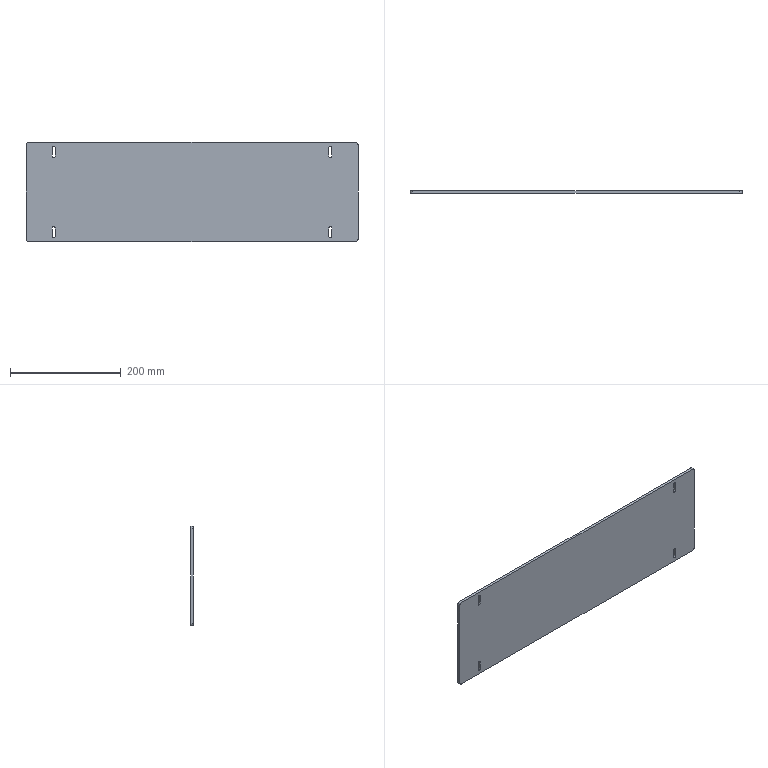Part | STEP file | H_ND24021-01-JG-098-TL | 1 solid | 30 faces | box 600 x 5 x 180 mm | volume 537768 mm3 | cylinder 16 | plane 14 | commonest cylinder face diameters 5.5 x12 10 x4